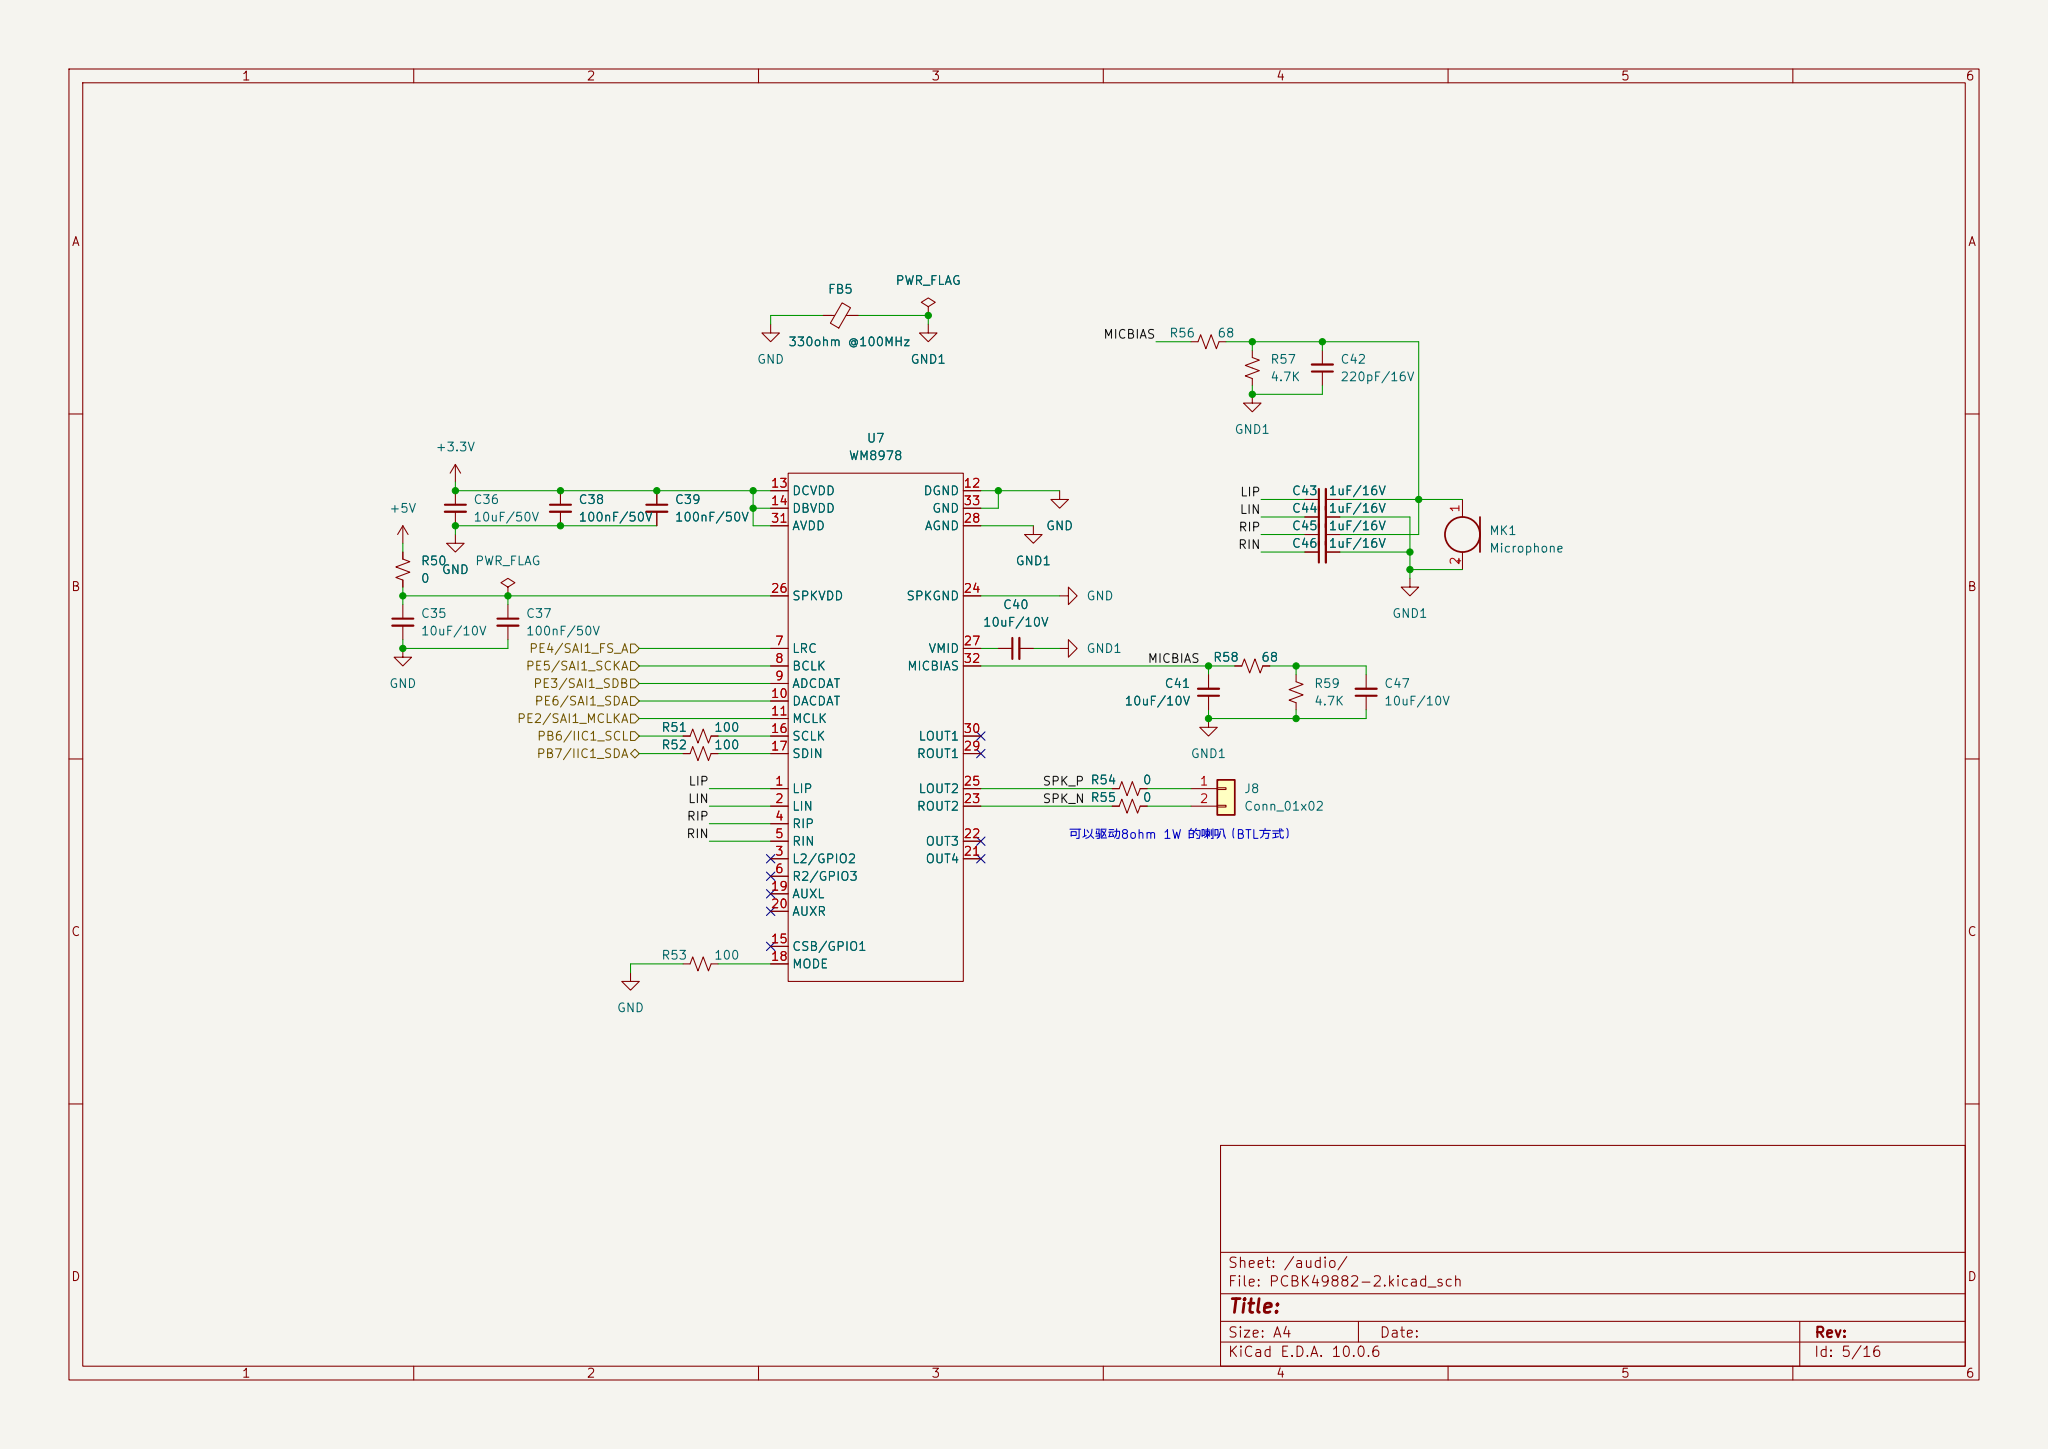Circuit board | KiCad | 536 parts | 438 nets | one sheet of the schematic
Parts on this sheet (reference | value | footprint):
C36 | 10uF/50V | Capacitor_SMD:C_0603_1608Metric
C37
C38
C39
C40 | 10uF/10V | Capacitor_SMD:C_0603_1608Metric
C41 | 10uF/10V | Capacitor_SMD:C_0603_1608Metric
C42 | 220pF/16V | Capacitor_SMD:C_0603_1608Metric
C43
C44
C45
C46
C47 | 10uF/10V | Capacitor_SMD:C_0603_1608Metric
FB5
MK1 | Microphone | Connector_User:MIC-TH_BD4.5-P1.60-D0.40-L-FD
R50 | 0 | Resistor_SMD:R_0603_1608Metric
R51
R52
R53
R54 | 0 | Resistor_SMD:R_0603_1608Metric
R55 | 0 | Resistor_SMD:R_0603_1608Metric
R56 | 68 | Resistor_SMD:R_0603_1608Metric
R57 | 4.7K | Resistor_SMD:R_0603_1608Metric
R58 | 68 | Resistor_SMD:R_0603_1608Metric
R59 | 4.7K | Resistor_SMD:R_0603_1608Metric
U7 | WM8978 | Package_DFN_QFN:QFN-32-1EP_5x5mm_P0.5mm_EP3.45x3.45mm
Nets of these parts (net: part-pin ...):
+3.3V: C36-1 C38-1 C39-1 U7-13 U7-14 U7-31
+5V: R50-1
/audio/LIN: C44-1 U7-2
/audio/LIP: C43-1 U7-1
/audio/MICBIAS: C41-2 R56-1 R58-1 U7-32
/audio/PB6{slash}IIC1_SCL: R51-1
/audio/PB7{slash}IIC1_SDA: R52-1
/audio/RIN: C46-1 U7-5
/audio/RIP: C45-1 U7-4
/audio/SPK_N: R55-1 U7-23
/audio/SPK_P: R54-1 U7-25
GND: C36-2 C37-2 C38-2 C39-2 FB5-1 R53-1 U7-12 U7-24 U7-33
GND1: C40-2 C41-1 C42-1 C44-2 C46-2 C47-1 FB5-2 MK1-2 R57-2 R59-2 U7-28
Net-(C47-Pad2): C47-2 R58-2 R59-1
Net-(J8-Pin_1): R54-2
Net-(J8-Pin_2): R55-2
Net-(MK1--): C42-2 C43-2 C45-2 MK1-1 R56-2 R57-1
Net-(U7-MODE): R53-2 U7-18
Net-(U7-SCLK): R51-2 U7-16
Net-(U7-SDIN): R52-2 U7-17
Net-(U7-SPKVDD): C37-1 R50-2 U7-26
Net-(U7-VMID): C40-1 U7-27